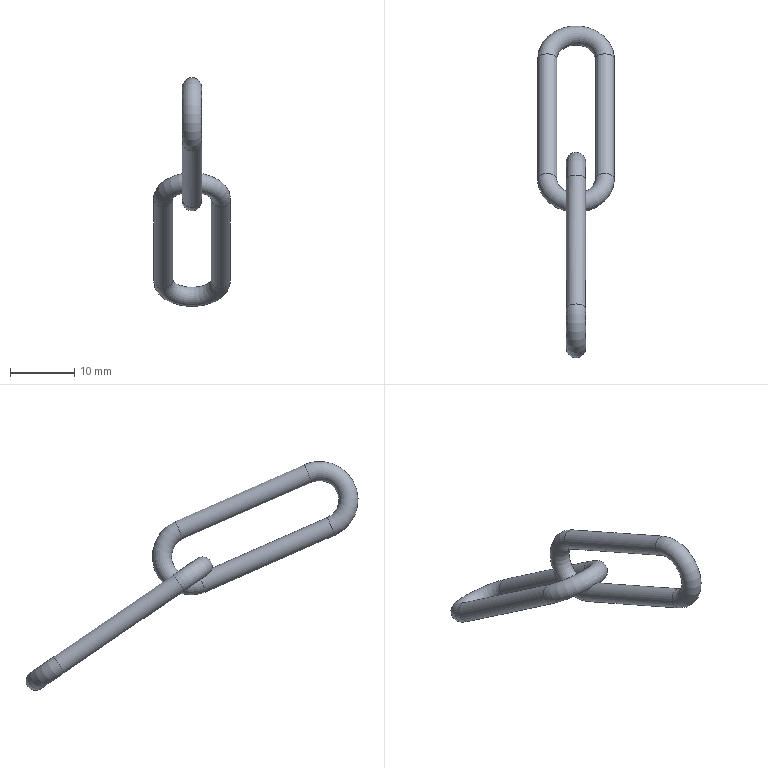Part | NX | features ACO1606-1-04.2 2 | 1 solid | 8 faces | box 12 x 51.907 x 35.782 mm | volume 1029 mm3 | torus 4 | cylinder 4 | commonest cylinder face diameters 3 x4
STEP:
#1=CARTESIAN_POINT('',(858.667,-815.544,-165.282));
#2=VERTEX_POINT('',#1);
#3=CARTESIAN_POINT('',(860.167,-815.544,-165.282));
#4=DIRECTION('',(0.,0.8254,-0.5645));
#5=DIRECTION('',(-1.,0.,0.));
#6=AXIS2_PLACEMENT_3D('',#3,#4,#5);
#7=CIRCLE('',#6,1.5);
#8=EDGE_CURVE('',#2,#2,#7,.T.);
#9=ORIENTED_EDGE('',*,*,#8,.F.);
#10=EDGE_LOOP('',(#9));
#11=FACE_BOUND('',#10,.T.);
#12=CARTESIAN_POINT('',(867.667,-815.544,-165.282));
#13=VERTEX_POINT('',#12);
#14=CARTESIAN_POINT('',(869.167,-815.544,-165.282));
#15=DIRECTION('',(0.,-0.8254,0.5645));
#16=DIRECTION('',(-1.,0.,0.));
#17=AXIS2_PLACEMENT_3D('',#14,#15,#16);
#18=CIRCLE('',#17,1.5);
#19=EDGE_CURVE('',#13,#13,#18,.T.);
#20=ORIENTED_EDGE('',*,*,#19,.T.);
#21=EDGE_LOOP('',(#20));
#22=FACE_BOUND('',#21,.T.);
#23=CARTESIAN_POINT('',(865.673,-818.751,-164.28));
#24=VERTEX_POINT('',#23);
#25=CARTESIAN_POINT('',(863.661,-818.751,-164.28));
#26=VERTEX_POINT('',#25);
#27=CARTESIAN_POINT('',(865.673,-818.751,-164.28));
#28=CARTESIAN_POINT('',(865.431,-818.482,-164.158));
#29=CARTESIAN_POINT('',(864.667,-818.376,-163.826));
#30=CARTESIAN_POINT('',(863.903,-818.482,-164.158));
#31=CARTESIAN_POINT('',(863.661,-818.751,-164.28));
#32=B_SPLINE_CURVE_WITH_KNOTS('',3,(#27,#28,#29,#30,#31),.UNSPECIFIED.,.F.,.F.,(4,1,4),(0.,0.001129,0.002258),.UNSPECIFIED.);
#33=EDGE_CURVE('',#24,#26,#32,.T.);
#34=ORIENTED_EDGE('',*,*,#33,.T.);
#35=CARTESIAN_POINT('',(863.661,-818.751,-164.28));
#36=CARTESIAN_POINT('',(863.479,-818.952,-164.371));
#37=CARTESIAN_POINT('',(863.346,-819.551,-164.378));
#38=CARTESIAN_POINT('',(863.418,-820.281,-163.886));
#39=CARTESIAN_POINT('',(863.822,-820.682,-163.209));
#40=CARTESIAN_POINT('',(864.665,-820.767,-162.872));
#41=CARTESIAN_POINT('',(865.509,-820.684,-163.205));
#42=CARTESIAN_POINT('',(865.917,-820.281,-163.886));
#43=CARTESIAN_POINT('',(865.988,-819.554,-164.377));
#44=CARTESIAN_POINT('',(865.855,-818.953,-164.371));
#45=CARTESIAN_POINT('',(865.673,-818.751,-164.28));
#46=B_SPLINE_CURVE_WITH_KNOTS('',3,(#35,#36,#37,#38,#39,#40,#41,#42,#43,#44,#45),.UNSPECIFIED.,.F.,.F.,(4,1,1,1,1,1,1,1,4),(0.,0.0008436,0.001687,0.002531,0.003374,0.004218,0.005061,0.005905,0.006748),.UNSPECIFIED.);
#47=EDGE_CURVE('',#26,#24,#46,.T.);
#48=ORIENTED_EDGE('',*,*,#47,.T.);
#49=EDGE_LOOP('',(#34,#48));
#50=FACE_BOUND('',#49,.T.);
#51=CARTESIAN_POINT('',(864.667,-815.544,-165.282));
#52=DIRECTION('',(0.,-0.5645,-0.8254));
#53=DIRECTION('',(0.,-0.8254,0.5645));
#54=AXIS2_PLACEMENT_3D('',#51,#52,#53);
#55=TOROIDAL_SURFACE('',#54,4.5,1.5);
#56=ADVANCED_FACE('',(#11,#22,#50),#55,.T.);
#57=CARTESIAN_POINT('',(867.667,-796.84,-178.074));
#58=VERTEX_POINT('',#57);
#59=CARTESIAN_POINT('',(869.167,-796.84,-178.074));
#60=DIRECTION('',(0.,-0.8254,0.5645));
#61=DIRECTION('',(-1.,0.,0.));
#62=AXIS2_PLACEMENT_3D('',#59,#60,#61);
#63=CIRCLE('',#62,1.5);
#64=EDGE_CURVE('',#58,#58,#63,.T.);
#65=ORIENTED_EDGE('',*,*,#64,.T.);
#66=EDGE_LOOP('',(#65));
#67=FACE_BOUND('',#66,.T.);
#68=ORIENTED_EDGE('',*,*,#19,.F.);
#69=EDGE_LOOP('',(#68));
#70=FACE_BOUND('',#69,.T.);
#71=CARTESIAN_POINT('',(869.167,-806.192,-171.678));
#72=DIRECTION('',(0.,-0.8254,0.5645));
#73=DIRECTION('',(0.,0.5645,0.8254));
#74=AXIS2_PLACEMENT_3D('',#71,#72,#73);
#75=CYLINDRICAL_SURFACE('',#74,1.5);
#76=ADVANCED_FACE('',(#67,#70),#75,.T.);
#77=ORIENTED_EDGE('',*,*,#64,.F.);
#78=EDGE_LOOP('',(#77));
#79=FACE_BOUND('',#78,.T.);
#80=CARTESIAN_POINT('',(858.667,-796.84,-178.074));
#81=VERTEX_POINT('',#80);
#82=CARTESIAN_POINT('',(860.167,-796.84,-178.074));
#83=DIRECTION('',(0.,0.8254,-0.5645));
#84=DIRECTION('',(-1.,0.,0.));
#85=AXIS2_PLACEMENT_3D('',#82,#83,#84);
#86=CIRCLE('',#85,1.5);
#87=EDGE_CURVE('',#81,#81,#86,.T.);
#88=ORIENTED_EDGE('',*,*,#87,.T.);
#89=EDGE_LOOP('',(#88));
#90=FACE_BOUND('',#89,.T.);
#91=CARTESIAN_POINT('',(864.667,-796.84,-178.074));
#92=DIRECTION('',(0.,-0.5645,-0.8254));
#93=DIRECTION('',(0.,-0.8254,0.5645));
#94=AXIS2_PLACEMENT_3D('',#91,#92,#93);
#95=TOROIDAL_SURFACE('',#94,4.5,1.5);
#96=ADVANCED_FACE('',(#79,#90),#95,.T.);
#97=ORIENTED_EDGE('',*,*,#8,.T.);
#98=EDGE_LOOP('',(#97));
#99=FACE_BOUND('',#98,.T.);
#100=ORIENTED_EDGE('',*,*,#87,.F.);
#101=EDGE_LOOP('',(#100));
#102=FACE_BOUND('',#101,.T.);
#103=CARTESIAN_POINT('',(860.167,-806.192,-171.678));
#104=DIRECTION('',(0.,0.8254,-0.5645));
#105=DIRECTION('',(0.,-0.5645,-0.8254));
#106=AXIS2_PLACEMENT_3D('',#103,#104,#105);
#107=CYLINDRICAL_SURFACE('',#106,1.5);
#108=ADVANCED_FACE('',(#99,#102),#107,.T.);
#109=CARTESIAN_POINT('',(864.667,-836.327,-149.586));
#110=VERTEX_POINT('',#109);
#111=CARTESIAN_POINT('',(863.167,-835.723,-148.213));
#112=VERTEX_POINT('',#111);
#113=CARTESIAN_POINT('',(864.667,-835.723,-148.213));
#114=DIRECTION('',(0.,0.9156,-0.4021));
#115=DIRECTION('',(-1.,0.,0.));
#116=AXIS2_PLACEMENT_3D('',#113,#114,#115);
#117=CIRCLE('',#116,1.5);
#118=EDGE_CURVE('',#110,#112,#117,.T.);
#119=ORIENTED_EDGE('',*,*,#118,.F.);
#120=CARTESIAN_POINT('',(866.167,-835.723,-148.213));
#121=VERTEX_POINT('',#120);
#122=CARTESIAN_POINT('',(864.667,-835.723,-148.213));
#123=DIRECTION('',(0.,0.9156,-0.4021));
#124=DIRECTION('',(-1.,0.,0.));
#125=AXIS2_PLACEMENT_3D('',#122,#123,#124);
#126=CIRCLE('',#125,1.5);
#127=EDGE_CURVE('',#121,#110,#126,.T.);
#128=ORIENTED_EDGE('',*,*,#127,.F.);
#129=CARTESIAN_POINT('',(864.667,-835.12,-146.839));
#130=VERTEX_POINT('',#129);
#131=CARTESIAN_POINT('',(864.667,-835.723,-148.213));
#132=DIRECTION('',(0.,0.9156,-0.4021));
#133=DIRECTION('',(-1.,0.,0.));
#134=AXIS2_PLACEMENT_3D('',#131,#132,#133);
#135=CIRCLE('',#134,1.5);
#136=EDGE_CURVE('',#130,#121,#135,.T.);
#137=ORIENTED_EDGE('',*,*,#136,.F.);
#138=CARTESIAN_POINT('',(864.667,-835.723,-148.213));
#139=DIRECTION('',(0.,0.9156,-0.4021));
#140=DIRECTION('',(-1.,0.,0.));
#141=AXIS2_PLACEMENT_3D('',#138,#139,#140);
#142=CIRCLE('',#141,1.5);
#143=EDGE_CURVE('',#112,#130,#142,.T.);
#144=ORIENTED_EDGE('',*,*,#143,.F.);
#145=EDGE_LOOP('',(#119,#128,#137,#144));
#146=FACE_BOUND('',#145,.T.);
#147=CARTESIAN_POINT('',(864.667,-838.739,-155.08));
#148=VERTEX_POINT('',#147);
#149=CARTESIAN_POINT('',(864.667,-839.945,-157.826));
#150=VERTEX_POINT('',#149);
#151=CARTESIAN_POINT('',(864.667,-839.342,-156.453));
#152=DIRECTION('',(0.,-0.9156,0.4021));
#153=DIRECTION('',(-1.,0.,0.));
#154=AXIS2_PLACEMENT_3D('',#151,#152,#153);
#155=CIRCLE('',#154,1.5);
#156=EDGE_CURVE('',#148,#150,#155,.T.);
#157=ORIENTED_EDGE('',*,*,#156,.T.);
#158=CARTESIAN_POINT('',(866.167,-839.342,-156.453));
#159=VERTEX_POINT('',#158);
#160=CARTESIAN_POINT('',(864.667,-839.342,-156.453));
#161=DIRECTION('',(0.,-0.9156,0.4021));
#162=DIRECTION('',(-1.,0.,0.));
#163=AXIS2_PLACEMENT_3D('',#160,#161,#162);
#164=CIRCLE('',#163,1.5);
#165=EDGE_CURVE('',#150,#159,#164,.T.);
#166=ORIENTED_EDGE('',*,*,#165,.T.);
#167=CARTESIAN_POINT('',(864.667,-839.342,-156.453));
#168=DIRECTION('',(0.,-0.9156,0.4021));
#169=DIRECTION('',(-1.,0.,0.));
#170=AXIS2_PLACEMENT_3D('',#167,#168,#169);
#171=CIRCLE('',#170,1.5);
#172=EDGE_CURVE('',#159,#148,#171,.T.);
#173=ORIENTED_EDGE('',*,*,#172,.T.);
#174=EDGE_LOOP('',(#157,#166,#173));
#175=FACE_BOUND('',#174,.T.);
#176=CARTESIAN_POINT('',(864.667,-837.533,-152.333));
#177=DIRECTION('',(-1.,0.,0.));
#178=DIRECTION('',(0.,0.,-1.));
#179=AXIS2_PLACEMENT_3D('',#176,#177,#178);
#180=TOROIDAL_SURFACE('',#179,4.5,1.5);
#181=ADVANCED_FACE('',(#146,#175),#180,.T.);
#182=ORIENTED_EDGE('',*,*,#156,.F.);
#183=ORIENTED_EDGE('',*,*,#172,.F.);
#184=ORIENTED_EDGE('',*,*,#165,.F.);
#185=EDGE_LOOP('',(#182,#183,#184));
#186=FACE_BOUND('',#185,.T.);
#187=CARTESIAN_POINT('',(864.667,-819.199,-165.298));
#188=DIRECTION('',(0.,-0.9156,0.4021));
#189=DIRECTION('',(-1.,0.,0.));
#190=AXIS2_PLACEMENT_3D('',#187,#188,#189);
#191=CIRCLE('',#190,1.5);
#192=EDGE_CURVE('',#26,#24,#191,.T.);
#193=ORIENTED_EDGE('',*,*,#192,.T.);
#194=ORIENTED_EDGE('',*,*,#47,.F.);
#195=EDGE_LOOP('',(#193,#194));
#196=FACE_BOUND('',#195,.T.);
#197=CARTESIAN_POINT('',(864.667,-827.693,-161.569));
#198=DIRECTION('',(0.,-0.9156,0.4021));
#199=DIRECTION('',(0.,0.4021,0.9156));
#200=AXIS2_PLACEMENT_3D('',#197,#198,#199);
#201=CYLINDRICAL_SURFACE('',#200,1.5);
#202=ADVANCED_FACE('',(#186,#196),#201,.T.);
#203=CARTESIAN_POINT('',(863.167,-815.58,-157.058));
#204=VERTEX_POINT('',#203);
#205=CARTESIAN_POINT('',(864.667,-815.58,-157.058));
#206=DIRECTION('',(0.,0.9156,-0.4021));
#207=DIRECTION('',(-1.,0.,0.));
#208=AXIS2_PLACEMENT_3D('',#205,#206,#207);
#209=CIRCLE('',#208,1.5);
#210=EDGE_CURVE('',#204,#204,#209,.T.);
#211=ORIENTED_EDGE('',*,*,#210,.F.);
#212=EDGE_LOOP('',(#211));
#213=FACE_BOUND('',#212,.T.);
#214=ORIENTED_EDGE('',*,*,#143,.T.);
#215=ORIENTED_EDGE('',*,*,#136,.T.);
#216=ORIENTED_EDGE('',*,*,#127,.T.);
#217=ORIENTED_EDGE('',*,*,#118,.T.);
#218=EDGE_LOOP('',(#214,#215,#216,#217));
#219=FACE_BOUND('',#218,.T.);
#220=CARTESIAN_POINT('',(864.667,-827.229,-151.942));
#221=DIRECTION('',(0.,0.9156,-0.4021));
#222=DIRECTION('',(0.,-0.4021,-0.9156));
#223=AXIS2_PLACEMENT_3D('',#220,#221,#222);
#224=CYLINDRICAL_SURFACE('',#223,1.5);
#225=ADVANCED_FACE('',(#213,#219),#224,.T.);
#226=ORIENTED_EDGE('',*,*,#192,.F.);
#227=ORIENTED_EDGE('',*,*,#33,.F.);
#228=EDGE_LOOP('',(#226,#227));
#229=FACE_BOUND('',#228,.T.);
#230=ORIENTED_EDGE('',*,*,#210,.T.);
#231=EDGE_LOOP('',(#230));
#232=FACE_BOUND('',#231,.T.);
#233=CARTESIAN_POINT('',(864.667,-817.389,-161.178));
#234=DIRECTION('',(-1.,0.,0.));
#235=DIRECTION('',(0.,0.,-1.));
#236=AXIS2_PLACEMENT_3D('',#233,#234,#235);
#237=TOROIDAL_SURFACE('',#236,4.5,1.5);
#238=ADVANCED_FACE('',(#229,#232),#237,.T.);
#239=CLOSED_SHELL('',(#56,#76,#96,#108,#181,#202,#225,#238));
#240=MANIFOLD_SOLID_BREP('',#239);
#241=(LENGTH_UNIT()NAMED_UNIT(*)SI_UNIT(.MILLI.,.METRE.));
#242=UNCERTAINTY_MEASURE_WITH_UNIT(LENGTH_MEASURE(0.0508),#241,'','');
#243=(NAMED_UNIT(*)PLANE_ANGLE_UNIT()SI_UNIT($,.RADIAN.));
#244=(NAMED_UNIT(*)SI_UNIT($,.STERADIAN.)SOLID_ANGLE_UNIT());
#245=(GEOMETRIC_REPRESENTATION_CONTEXT(3)GLOBAL_UNCERTAINTY_ASSIGNED_CONTEXT((#242))GLOBAL_UNIT_ASSIGNED_CONTEXT((#241,#243,#244))REPRESENTATION_CONTEXT('',''));
#246=ADVANCED_BREP_SHAPE_REPRESENTATION('',(#240),#245);